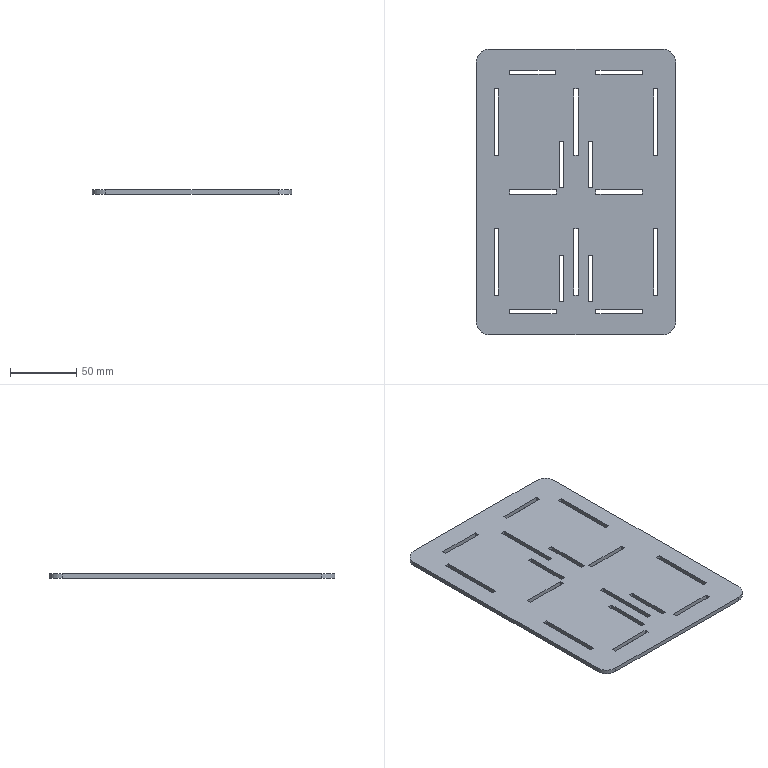Part | SolidWorks | features FlatPattern 1, SMBaseFlange 1, SheetMetal 1 | 1 solid | 74 faces | box 150 x 215 x 3.2 mm | volume 96275 mm3 | plane 70 | cylinder 4 | commonest cylinder face diameters 20 x4